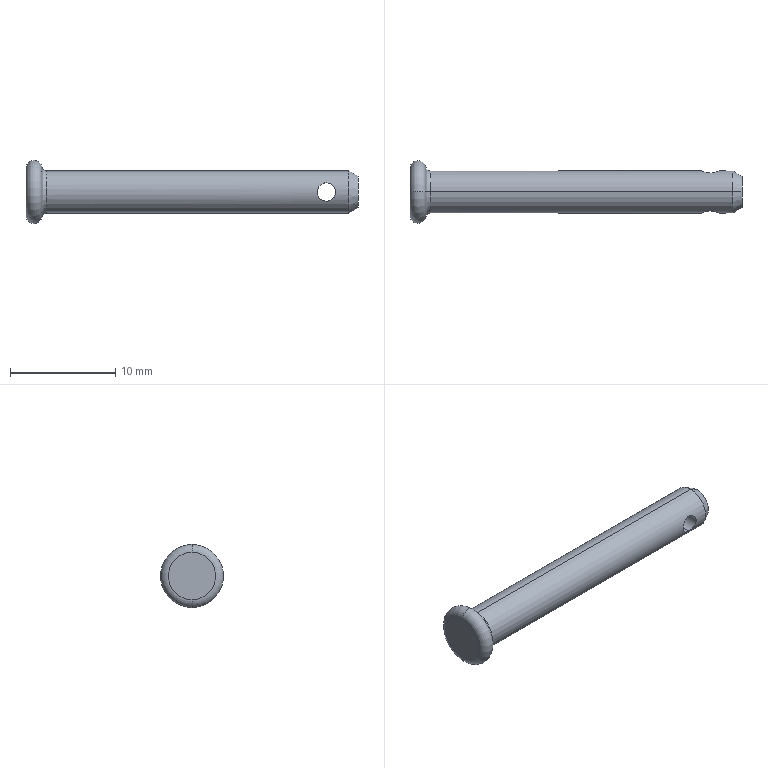Part | SolidWorks | features Chamfer 1, Cut 1, Fillet 1, Revolution 1 | 1 solid | 12 faces | box 31.5 x 6 x 6 mm | volume 403.91 mm3 | cylinder 4 | torus 4 | cone 2 | plane 2 | commonest cylinder face diameters 1.74 x2 4 x2
STEP:
#1=CARTESIAN_POINT('',(28.5,-1.801,-0.87));
#2=VERTEX_POINT('',#1);
#3=CARTESIAN_POINT('',(28.5,-1.801,0.87));
#4=VERTEX_POINT('',#3);
#5=CARTESIAN_POINT('',(28.5,-1.801,-0.87));
#6=CARTESIAN_POINT('',(28.385,-1.801,-0.87));
#7=CARTESIAN_POINT('',(28.27,-1.813,-0.8468));
#8=CARTESIAN_POINT('',(28.059,-1.851,-0.7588));
#9=CARTESIAN_POINT('',(27.964,-1.877,-0.6948));
#10=CARTESIAN_POINT('',(27.805,-1.929,-0.5353));
#11=CARTESIAN_POINT('',(27.741,-1.954,-0.4401));
#12=CARTESIAN_POINT('',(27.653,-1.99,-0.2304));
#13=CARTESIAN_POINT('',(27.63,-2.,-0.115));
#14=CARTESIAN_POINT('',(27.63,-2.,0.1145));
#15=CARTESIAN_POINT('',(27.653,-1.99,0.2302));
#16=CARTESIAN_POINT('',(27.741,-1.954,0.4402));
#17=CARTESIAN_POINT('',(27.805,-1.929,0.5355));
#18=CARTESIAN_POINT('',(28.045,-1.851,0.7751));
#19=CARTESIAN_POINT('',(28.267,-1.801,0.87));
#20=CARTESIAN_POINT('',(28.5,-1.801,0.87));
#21=B_SPLINE_CURVE_WITH_KNOTS('',3,(#5,#6,#7,#8,#9,#10,#11,#12,#13,#14,#15,#16,#17,#18,#19,#20),.UNSPECIFIED.,.F.,.F.,(4,2,2,2,2,2,2,4),(0.002755,0.003099,0.003443,0.003787,0.004131,0.004475,0.004819,0.005507),.UNSPECIFIED.);
#22=EDGE_CURVE('',#2,#4,#21,.T.);
#23=ORIENTED_EDGE('',*,*,#22,.F.);
#24=CARTESIAN_POINT('',(28.5,1.801,-0.87));
#25=VERTEX_POINT('',#24);
#26=CARTESIAN_POINT('',(28.5,-500.,-0.87));
#27=DIRECTION('',(0.,1.,0.));
#28=VECTOR('',#27,1000.);
#29=LINE('',#26,#28);
#30=EDGE_CURVE('',#2,#25,#29,.T.);
#31=ORIENTED_EDGE('',*,*,#30,.T.);
#32=CARTESIAN_POINT('',(28.5,1.801,0.87));
#33=VERTEX_POINT('',#32);
#34=CARTESIAN_POINT('',(28.5,1.801,0.87));
#35=CARTESIAN_POINT('',(28.383,1.801,0.87));
#36=CARTESIAN_POINT('',(28.269,1.813,0.8465));
#37=CARTESIAN_POINT('',(28.059,1.851,0.7588));
#38=CARTESIAN_POINT('',(27.964,1.877,0.6944));
#39=CARTESIAN_POINT('',(27.806,1.929,0.536));
#40=CARTESIAN_POINT('',(27.741,1.954,0.4402));
#41=CARTESIAN_POINT('',(27.654,1.989,0.2311));
#42=CARTESIAN_POINT('',(27.63,2.,0.1157));
#43=CARTESIAN_POINT('',(27.63,2.,-0.1148));
#44=CARTESIAN_POINT('',(27.653,1.99,-0.2298));
#45=CARTESIAN_POINT('',(27.742,1.954,-0.4417));
#46=CARTESIAN_POINT('',(27.806,1.928,-0.5366));
#47=CARTESIAN_POINT('',(27.965,1.877,-0.6952));
#48=CARTESIAN_POINT('',(28.061,1.851,-0.7594));
#49=CARTESIAN_POINT('',(28.269,1.813,-0.8465));
#50=CARTESIAN_POINT('',(28.385,1.801,-0.87));
#51=CARTESIAN_POINT('',(28.5,1.801,-0.87));
#52=B_SPLINE_CURVE_WITH_KNOTS('',3,(#34,#35,#36,#37,#38,#39,#40,#41,#42,#43,#44,#45,#46,#47,#48,#49,#50,#51),.UNSPECIFIED.,.F.,.F.,(4,2,2,2,2,2,2,2,4),(0.,0.0003443,0.0006887,0.001033,0.001377,0.001722,0.002066,0.00241,0.002755),.UNSPECIFIED.);
#53=EDGE_CURVE('',#33,#25,#52,.T.);
#54=ORIENTED_EDGE('',*,*,#53,.F.);
#55=CARTESIAN_POINT('',(28.5,-500.,0.87));
#56=DIRECTION('',(0.,1.,0.));
#57=VECTOR('',#56,1000.);
#58=LINE('',#55,#57);
#59=EDGE_CURVE('',#4,#33,#58,.T.);
#60=ORIENTED_EDGE('',*,*,#59,.F.);
#61=EDGE_LOOP('',(#23,#31,#54,#60));
#62=FACE_OUTER_BOUND('',#61,.T.);
#63=CARTESIAN_POINT('',(28.5,-500.,0.));
#64=DIRECTION('',(0.,1.,0.));
#65=DIRECTION('',(0.,0.,1.));
#66=AXIS2_PLACEMENT_3D('',#63,#64,#65);
#67=CYLINDRICAL_SURFACE('',#66,0.87);
#68=ADVANCED_FACE('',(#62),#67,.F.);
#69=CARTESIAN_POINT('',(31.5,0.,-1.5));
#70=VERTEX_POINT('',#69);
#71=CARTESIAN_POINT('',(31.5,0.,1.5));
#72=VERTEX_POINT('',#71);
#73=CARTESIAN_POINT('',(31.5,0.,0.));
#74=DIRECTION('',(1.,0.,0.));
#75=DIRECTION('',(0.,0.,1.));
#76=AXIS2_PLACEMENT_3D('',#73,#74,#75);
#77=CIRCLE('',#76,1.5);
#78=EDGE_CURVE('',#70,#72,#77,.T.);
#79=ORIENTED_EDGE('',*,*,#78,.F.);
#80=CARTESIAN_POINT('',(30.634,0.,-2.));
#81=VERTEX_POINT('',#80);
#82=CARTESIAN_POINT('',(30.634,0.,-2.));
#83=DIRECTION('',(-0.866,0.,-0.5));
#84=VECTOR('',#83,1000.);
#85=LINE('',#82,#84);
#86=EDGE_CURVE('',#70,#81,#85,.T.);
#87=ORIENTED_EDGE('',*,*,#86,.T.);
#88=CARTESIAN_POINT('',(30.634,0.,2.));
#89=VERTEX_POINT('',#88);
#90=CARTESIAN_POINT('',(30.634,0.,0.));
#91=DIRECTION('',(-1.,0.,0.));
#92=DIRECTION('',(0.,0.,1.));
#93=AXIS2_PLACEMENT_3D('',#90,#91,#92);
#94=CIRCLE('',#93,2.);
#95=EDGE_CURVE('',#89,#81,#94,.T.);
#96=ORIENTED_EDGE('',*,*,#95,.F.);
#97=CARTESIAN_POINT('',(30.634,0.,2.));
#98=DIRECTION('',(-0.866,0.,0.5));
#99=VECTOR('',#98,1000.);
#100=LINE('',#97,#99);
#101=EDGE_CURVE('',#72,#89,#100,.T.);
#102=ORIENTED_EDGE('',*,*,#101,.F.);
#103=EDGE_LOOP('',(#79,#87,#96,#102));
#104=FACE_OUTER_BOUND('',#103,.T.);
#105=CARTESIAN_POINT('',(30.634,0.,0.));
#106=DIRECTION('',(-1.,0.,0.));
#107=DIRECTION('',(0.,0.,1.));
#108=AXIS2_PLACEMENT_3D('',#105,#106,#107);
#109=CONICAL_SURFACE('',#108,2.,0.5236);
#110=ADVANCED_FACE('',(#104),#109,.T.);
#111=CARTESIAN_POINT('',(1.485,0.,-2.4));
#112=VERTEX_POINT('',#111);
#113=CARTESIAN_POINT('',(1.485,0.,2.4));
#114=VERTEX_POINT('',#113);
#115=CARTESIAN_POINT('',(1.485,0.,0.));
#116=DIRECTION('',(-1.,0.,0.));
#117=DIRECTION('',(0.,0.,1.));
#118=AXIS2_PLACEMENT_3D('',#115,#116,#117);
#119=CIRCLE('',#118,2.4);
#120=EDGE_CURVE('',#112,#114,#119,.T.);
#121=ORIENTED_EDGE('',*,*,#120,.F.);
#122=CARTESIAN_POINT('',(1.975,0.,-2.));
#123=VERTEX_POINT('',#122);
#124=CARTESIAN_POINT('',(1.975,0.,-2.5));
#125=DIRECTION('',(0.,1.,0.));
#126=DIRECTION('',(0.,0.,1.));
#127=AXIS2_PLACEMENT_3D('',#124,#125,#126);
#128=CIRCLE('',#127,0.5);
#129=EDGE_CURVE('',#112,#123,#128,.T.);
#130=ORIENTED_EDGE('',*,*,#129,.T.);
#131=CARTESIAN_POINT('',(1.975,0.,2.));
#132=VERTEX_POINT('',#131);
#133=CARTESIAN_POINT('',(1.975,0.,0.));
#134=DIRECTION('',(1.,0.,0.));
#135=DIRECTION('',(0.,0.,1.));
#136=AXIS2_PLACEMENT_3D('',#133,#134,#135);
#137=CIRCLE('',#136,2.);
#138=EDGE_CURVE('',#132,#123,#137,.T.);
#139=ORIENTED_EDGE('',*,*,#138,.F.);
#140=CARTESIAN_POINT('',(1.975,0.,2.5));
#141=DIRECTION('',(0.,-1.,0.));
#142=DIRECTION('',(0.,0.,-1.));
#143=AXIS2_PLACEMENT_3D('',#140,#141,#142);
#144=CIRCLE('',#143,0.5);
#145=EDGE_CURVE('',#114,#132,#144,.T.);
#146=ORIENTED_EDGE('',*,*,#145,.F.);
#147=EDGE_LOOP('',(#121,#130,#139,#146));
#148=FACE_OUTER_BOUND('',#147,.T.);
#149=CARTESIAN_POINT('',(1.975,0.,0.));
#150=DIRECTION('',(-1.,0.,0.));
#151=DIRECTION('',(0.,0.,1.));
#152=AXIS2_PLACEMENT_3D('',#149,#150,#151);
#153=TOROIDAL_SURFACE('',#152,2.5,0.5);
#154=ADVANCED_FACE('',(#148),#153,.F.);
#155=ORIENTED_EDGE('',*,*,#53,.T.);
#156=CARTESIAN_POINT('',(28.5,1.801,-0.87));
#157=CARTESIAN_POINT('',(28.615,1.801,-0.87));
#158=CARTESIAN_POINT('',(28.73,1.813,-0.8468));
#159=CARTESIAN_POINT('',(28.941,1.851,-0.7588));
#160=CARTESIAN_POINT('',(29.036,1.877,-0.6948));
#161=CARTESIAN_POINT('',(29.195,1.929,-0.5353));
#162=CARTESIAN_POINT('',(29.259,1.954,-0.4401));
#163=CARTESIAN_POINT('',(29.347,1.99,-0.2304));
#164=CARTESIAN_POINT('',(29.37,2.,-0.115));
#165=CARTESIAN_POINT('',(29.37,2.,0.1145));
#166=CARTESIAN_POINT('',(29.347,1.99,0.2302));
#167=CARTESIAN_POINT('',(29.259,1.954,0.4402));
#168=CARTESIAN_POINT('',(29.195,1.929,0.5355));
#169=CARTESIAN_POINT('',(28.955,1.851,0.7751));
#170=CARTESIAN_POINT('',(28.733,1.801,0.87));
#171=CARTESIAN_POINT('',(28.5,1.801,0.87));
#172=B_SPLINE_CURVE_WITH_KNOTS('',3,(#156,#157,#158,#159,#160,#161,#162,#163,#164,#165,#166,#167,#168,#169,#170,#171),.UNSPECIFIED.,.F.,.F.,(4,2,2,2,2,2,2,4),(0.002755,0.003099,0.003443,0.003787,0.004131,0.004475,0.004819,0.005507),.UNSPECIFIED.);
#173=EDGE_CURVE('',#25,#33,#172,.T.);
#174=ORIENTED_EDGE('',*,*,#173,.T.);
#175=EDGE_LOOP('',(#155,#174));
#176=FACE_BOUND('',#175,.T.);
#177=ORIENTED_EDGE('',*,*,#95,.T.);
#178=CARTESIAN_POINT('',(0.,0.,-2.));
#179=DIRECTION('',(-1.,0.,0.));
#180=VECTOR('',#179,1000.);
#181=LINE('',#178,#180);
#182=EDGE_CURVE('',#81,#123,#181,.T.);
#183=ORIENTED_EDGE('',*,*,#182,.T.);
#184=CARTESIAN_POINT('',(1.975,0.,0.));
#185=DIRECTION('',(1.,0.,0.));
#186=DIRECTION('',(0.,0.,1.));
#187=AXIS2_PLACEMENT_3D('',#184,#185,#186);
#188=CIRCLE('',#187,2.);
#189=EDGE_CURVE('',#123,#132,#188,.T.);
#190=ORIENTED_EDGE('',*,*,#189,.T.);
#191=CARTESIAN_POINT('',(0.,0.,2.));
#192=DIRECTION('',(-1.,0.,0.));
#193=VECTOR('',#192,1000.);
#194=LINE('',#191,#193);
#195=EDGE_CURVE('',#89,#132,#194,.T.);
#196=ORIENTED_EDGE('',*,*,#195,.F.);
#197=EDGE_LOOP('',(#177,#183,#190,#196));
#198=FACE_OUTER_BOUND('',#197,.T.);
#199=CARTESIAN_POINT('',(0.,0.,0.));
#200=DIRECTION('',(-1.,0.,0.));
#201=DIRECTION('',(0.,0.,1.));
#202=AXIS2_PLACEMENT_3D('',#199,#200,#201);
#203=CYLINDRICAL_SURFACE('',#202,2.);
#204=ADVANCED_FACE('',(#176,#198),#203,.T.);
#205=CARTESIAN_POINT('',(1.485,0.,0.));
#206=DIRECTION('',(-1.,0.,0.));
#207=DIRECTION('',(0.,0.,1.));
#208=AXIS2_PLACEMENT_3D('',#205,#206,#207);
#209=CIRCLE('',#208,2.4);
#210=EDGE_CURVE('',#114,#112,#209,.T.);
#211=ORIENTED_EDGE('',*,*,#210,.T.);
#212=CARTESIAN_POINT('',(0.,0.,-2.25));
#213=VERTEX_POINT('',#212);
#214=CARTESIAN_POINT('',(0.75,0.,-2.25));
#215=DIRECTION('',(0.,1.,0.));
#216=DIRECTION('',(0.,0.,1.));
#217=AXIS2_PLACEMENT_3D('',#214,#215,#216);
#218=CIRCLE('',#217,0.75);
#219=EDGE_CURVE('',#112,#213,#218,.T.);
#220=ORIENTED_EDGE('',*,*,#219,.T.);
#221=CARTESIAN_POINT('',(0.,0.,2.25));
#222=VERTEX_POINT('',#221);
#223=CARTESIAN_POINT('',(0.,0.,0.));
#224=DIRECTION('',(-1.,0.,0.));
#225=DIRECTION('',(0.,0.,1.));
#226=AXIS2_PLACEMENT_3D('',#223,#224,#225);
#227=CIRCLE('',#226,2.25);
#228=EDGE_CURVE('',#222,#213,#227,.T.);
#229=ORIENTED_EDGE('',*,*,#228,.F.);
#230=CARTESIAN_POINT('',(0.75,0.,2.25));
#231=DIRECTION('',(0.,-1.,0.));
#232=DIRECTION('',(0.,0.,-1.));
#233=AXIS2_PLACEMENT_3D('',#230,#231,#232);
#234=CIRCLE('',#233,0.75);
#235=EDGE_CURVE('',#114,#222,#234,.T.);
#236=ORIENTED_EDGE('',*,*,#235,.F.);
#237=EDGE_LOOP('',(#211,#220,#229,#236));
#238=FACE_OUTER_BOUND('',#237,.T.);
#239=CARTESIAN_POINT('',(0.75,0.,0.));
#240=DIRECTION('',(-1.,0.,0.));
#241=DIRECTION('',(0.,0.,1.));
#242=AXIS2_PLACEMENT_3D('',#239,#240,#241);
#243=TOROIDAL_SURFACE('',#242,2.25,0.75);
#244=ADVANCED_FACE('',(#238),#243,.T.);
#245=ORIENTED_EDGE('',*,*,#228,.T.);
#246=CARTESIAN_POINT('',(0.,0.,0.));
#247=DIRECTION('',(-1.,0.,0.));
#248=DIRECTION('',(0.,0.,1.));
#249=AXIS2_PLACEMENT_3D('',#246,#247,#248);
#250=CIRCLE('',#249,2.25);
#251=EDGE_CURVE('',#213,#222,#250,.T.);
#252=ORIENTED_EDGE('',*,*,#251,.T.);
#253=EDGE_LOOP('',(#245,#252));
#254=FACE_OUTER_BOUND('',#253,.T.);
#255=CARTESIAN_POINT('',(0.,0.,0.));
#256=DIRECTION('',(1.,0.,0.));
#257=DIRECTION('',(0.,0.,-1.));
#258=AXIS2_PLACEMENT_3D('',#255,#256,#257);
#259=PLANE('',#258);
#260=ADVANCED_FACE('',(#254),#259,.F.);
#261=ORIENTED_EDGE('',*,*,#219,.F.);
#262=ORIENTED_EDGE('',*,*,#120,.T.);
#263=ORIENTED_EDGE('',*,*,#235,.T.);
#264=ORIENTED_EDGE('',*,*,#251,.F.);
#265=EDGE_LOOP('',(#261,#262,#263,#264));
#266=FACE_OUTER_BOUND('',#265,.T.);
#267=CARTESIAN_POINT('',(0.75,0.,0.));
#268=DIRECTION('',(-1.,0.,0.));
#269=DIRECTION('',(0.,0.,1.));
#270=AXIS2_PLACEMENT_3D('',#267,#268,#269);
#271=TOROIDAL_SURFACE('',#270,2.25,0.75);
#272=ADVANCED_FACE('',(#266),#271,.T.);
#273=ORIENTED_EDGE('',*,*,#182,.F.);
#274=CARTESIAN_POINT('',(30.634,0.,0.));
#275=DIRECTION('',(-1.,0.,0.));
#276=DIRECTION('',(0.,0.,1.));
#277=AXIS2_PLACEMENT_3D('',#274,#275,#276);
#278=CIRCLE('',#277,2.);
#279=EDGE_CURVE('',#81,#89,#278,.T.);
#280=ORIENTED_EDGE('',*,*,#279,.T.);
#281=ORIENTED_EDGE('',*,*,#195,.T.);
#282=ORIENTED_EDGE('',*,*,#138,.T.);
#283=EDGE_LOOP('',(#273,#280,#281,#282));
#284=FACE_OUTER_BOUND('',#283,.T.);
#285=CARTESIAN_POINT('',(28.5,-1.801,0.87));
#286=CARTESIAN_POINT('',(28.617,-1.801,0.87));
#287=CARTESIAN_POINT('',(28.731,-1.813,0.8465));
#288=CARTESIAN_POINT('',(28.941,-1.851,0.7588));
#289=CARTESIAN_POINT('',(29.036,-1.877,0.6944));
#290=CARTESIAN_POINT('',(29.194,-1.929,0.536));
#291=CARTESIAN_POINT('',(29.259,-1.954,0.4402));
#292=CARTESIAN_POINT('',(29.346,-1.989,0.2311));
#293=CARTESIAN_POINT('',(29.37,-2.,0.1157));
#294=CARTESIAN_POINT('',(29.37,-2.,-0.1148));
#295=CARTESIAN_POINT('',(29.347,-1.99,-0.2298));
#296=CARTESIAN_POINT('',(29.258,-1.954,-0.4417));
#297=CARTESIAN_POINT('',(29.194,-1.928,-0.5366));
#298=CARTESIAN_POINT('',(29.035,-1.877,-0.6952));
#299=CARTESIAN_POINT('',(28.939,-1.851,-0.7594));
#300=CARTESIAN_POINT('',(28.731,-1.813,-0.8465));
#301=CARTESIAN_POINT('',(28.615,-1.801,-0.87));
#302=CARTESIAN_POINT('',(28.5,-1.801,-0.87));
#303=B_SPLINE_CURVE_WITH_KNOTS('',3,(#285,#286,#287,#288,#289,#290,#291,#292,#293,#294,#295,#296,#297,#298,#299,#300,#301,#302),.UNSPECIFIED.,.F.,.F.,(4,2,2,2,2,2,2,2,4),(0.,0.0003443,0.0006887,0.001033,0.001377,0.001722,0.002066,0.00241,0.002755),.UNSPECIFIED.);
#304=EDGE_CURVE('',#4,#2,#303,.T.);
#305=ORIENTED_EDGE('',*,*,#304,.T.);
#306=ORIENTED_EDGE('',*,*,#22,.T.);
#307=EDGE_LOOP('',(#305,#306));
#308=FACE_BOUND('',#307,.T.);
#309=CARTESIAN_POINT('',(0.,0.,0.));
#310=DIRECTION('',(-1.,0.,0.));
#311=DIRECTION('',(0.,0.,1.));
#312=AXIS2_PLACEMENT_3D('',#309,#310,#311);
#313=CYLINDRICAL_SURFACE('',#312,2.);
#314=ADVANCED_FACE('',(#284,#308),#313,.T.);
#315=CARTESIAN_POINT('',(31.5,0.,0.));
#316=DIRECTION('',(1.,0.,0.));
#317=DIRECTION('',(0.,0.,1.));
#318=AXIS2_PLACEMENT_3D('',#315,#316,#317);
#319=CIRCLE('',#318,1.5);
#320=EDGE_CURVE('',#72,#70,#319,.T.);
#321=ORIENTED_EDGE('',*,*,#320,.T.);
#322=ORIENTED_EDGE('',*,*,#78,.T.);
#323=EDGE_LOOP('',(#321,#322));
#324=FACE_OUTER_BOUND('',#323,.T.);
#325=CARTESIAN_POINT('',(31.5,2.,0.));
#326=DIRECTION('',(-1.,0.,0.));
#327=DIRECTION('',(0.,0.,1.));
#328=AXIS2_PLACEMENT_3D('',#325,#326,#327);
#329=PLANE('',#328);
#330=ADVANCED_FACE('',(#324),#329,.F.);
#331=ORIENTED_EDGE('',*,*,#129,.F.);
#332=ORIENTED_EDGE('',*,*,#210,.F.);
#333=ORIENTED_EDGE('',*,*,#145,.T.);
#334=ORIENTED_EDGE('',*,*,#189,.F.);
#335=EDGE_LOOP('',(#331,#332,#333,#334));
#336=FACE_OUTER_BOUND('',#335,.T.);
#337=CARTESIAN_POINT('',(1.975,0.,0.));
#338=DIRECTION('',(-1.,0.,0.));
#339=DIRECTION('',(0.,0.,1.));
#340=AXIS2_PLACEMENT_3D('',#337,#338,#339);
#341=TOROIDAL_SURFACE('',#340,2.5,0.5);
#342=ADVANCED_FACE('',(#336),#341,.F.);
#343=ORIENTED_EDGE('',*,*,#86,.F.);
#344=ORIENTED_EDGE('',*,*,#320,.F.);
#345=ORIENTED_EDGE('',*,*,#101,.T.);
#346=ORIENTED_EDGE('',*,*,#279,.F.);
#347=EDGE_LOOP('',(#343,#344,#345,#346));
#348=FACE_OUTER_BOUND('',#347,.T.);
#349=CARTESIAN_POINT('',(30.634,0.,0.));
#350=DIRECTION('',(-1.,0.,0.));
#351=DIRECTION('',(0.,0.,1.));
#352=AXIS2_PLACEMENT_3D('',#349,#350,#351);
#353=CONICAL_SURFACE('',#352,2.,0.5236);
#354=ADVANCED_FACE('',(#348),#353,.T.);
#355=ORIENTED_EDGE('',*,*,#30,.F.);
#356=ORIENTED_EDGE('',*,*,#304,.F.);
#357=ORIENTED_EDGE('',*,*,#59,.T.);
#358=ORIENTED_EDGE('',*,*,#173,.F.);
#359=EDGE_LOOP('',(#355,#356,#357,#358));
#360=FACE_OUTER_BOUND('',#359,.T.);
#361=CARTESIAN_POINT('',(28.5,-500.,0.));
#362=DIRECTION('',(0.,1.,0.));
#363=DIRECTION('',(0.,0.,1.));
#364=AXIS2_PLACEMENT_3D('',#361,#362,#363);
#365=CYLINDRICAL_SURFACE('',#364,0.87);
#366=ADVANCED_FACE('',(#360),#365,.F.);
#367=CLOSED_SHELL('',(#68,#110,#154,#204,#244,#260,#272,#314,#330,#342,#354,#366));
#368=MANIFOLD_SOLID_BREP('',#367);
#369=CARTESIAN_POINT('',(0.,0.,0.));
#370=DIRECTION('',(0.,0.,1.));
#371=DIRECTION('',(1.,0.,0.));
#372=AXIS2_PLACEMENT_3D('',#369,#370,#371);
#373=(LENGTH_UNIT()NAMED_UNIT(*)SI_UNIT(.MILLI.,.METRE.));
#374=UNCERTAINTY_MEASURE_WITH_UNIT(LENGTH_MEASURE(0.00001),#373,'','');
#375=(NAMED_UNIT(*)PLANE_ANGLE_UNIT()SI_UNIT($,.RADIAN.));
#376=(NAMED_UNIT(*)SI_UNIT($,.STERADIAN.)SOLID_ANGLE_UNIT());
#377=(GEOMETRIC_REPRESENTATION_CONTEXT(3)GLOBAL_UNCERTAINTY_ASSIGNED_CONTEXT((#374))GLOBAL_UNIT_ASSIGNED_CONTEXT((#373,#375,#376))REPRESENTATION_CONTEXT('',''));
#378=ADVANCED_BREP_SHAPE_REPRESENTATION('',(#368,#372),#377);